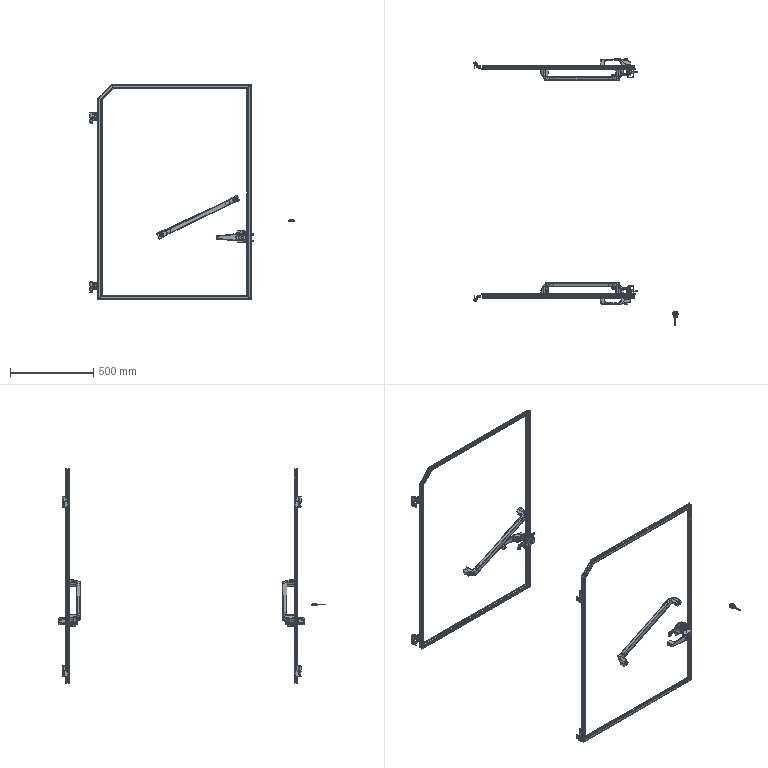Part | NX | features BREP 75 | 111 solids | 5675 faces | volume 1191779 mm3 | cylinder 2371 | plane 1729 | spline 913 | cone 345 | torus 243 | sphere 74 | commonest cylinder face diameters 6 x249 4 x238 2 x156 10 x156 2.56 x120 1 x115